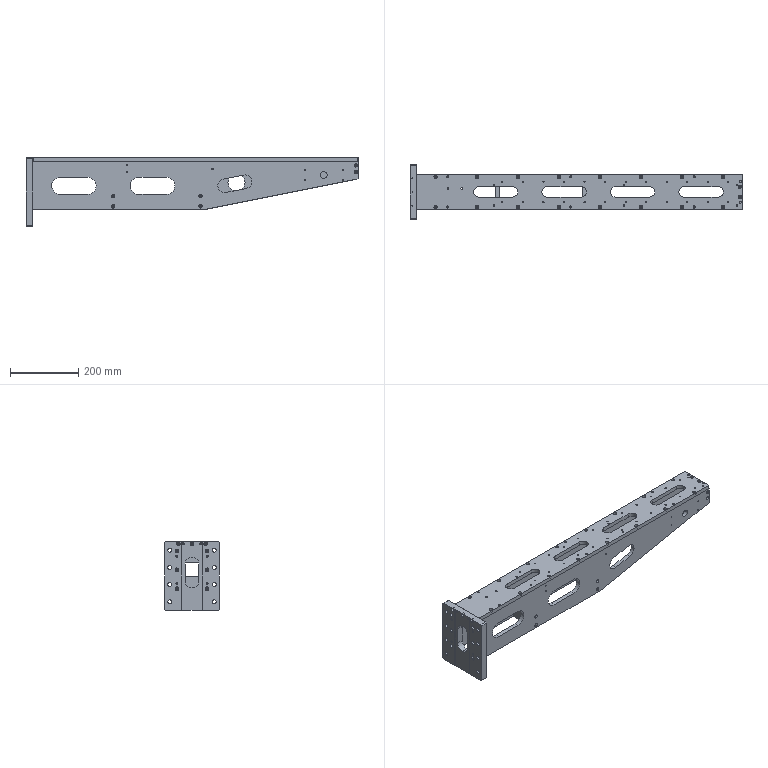Part | SolidWorks | features AEMSimFeature 1 | 7 solids | 705 faces | box 970 x 160 x 200 mm | volume 3941327 mm3 | cylinder 438 | cone 134 | plane 133 | commonest cylinder face diameters 3.3 x76 4.2 x60 5.5 x60 10 x60 6 x52 11 x34